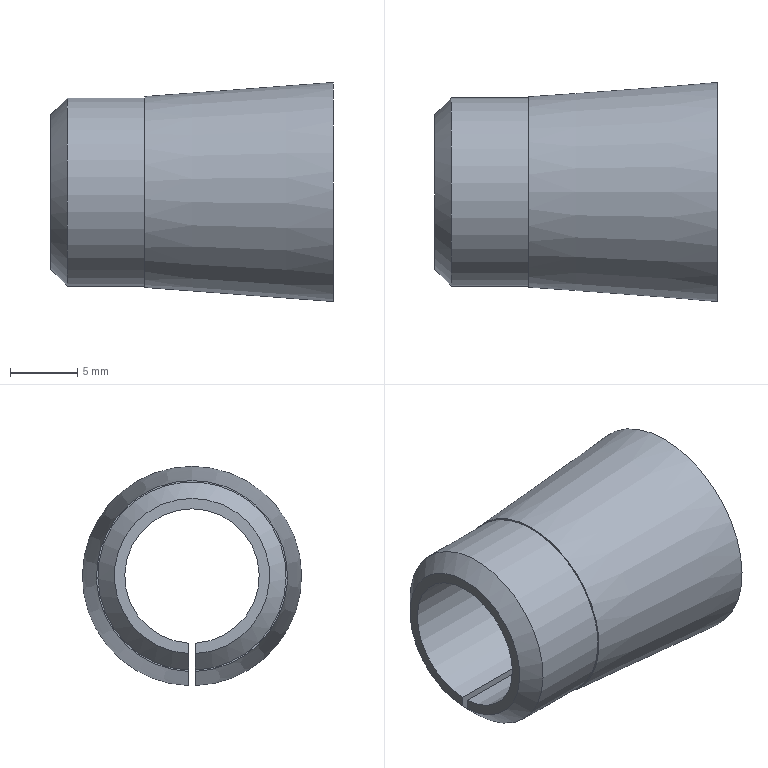Part | STEP file | 2_6 | 1 solid | 9 faces | box 21 x 16.3 x 16.296 mm | volume 1933 mm3 | plane 5 | cone 2 | cylinder 2 | commonest cylinder face diameters 10 x1 14 x1
STEP:
#1=CARTESIAN_POINT('',(0.,0.,0.));
#2=DIRECTION('',(0.,0.,1.));
#3=DIRECTION('',(1.,0.,0.));
#4=AXIS2_PLACEMENT_3D('',#1,#2,#3);
#5=CARTESIAN_POINT('',(7.,0.25,-7.096));
#6=VERTEX_POINT('',#5);
#7=CARTESIAN_POINT('',(7.,-0.25,-7.096));
#8=VERTEX_POINT('',#7);
#9=CARTESIAN_POINT('',(7.,0.,0.));
#10=DIRECTION('',(1.,0.,0.));
#11=DIRECTION('',(0.,0.,-1.));
#12=AXIS2_PLACEMENT_3D('',#9,#10,#11);
#13=CIRCLE('',#12,7.1);
#14=CARTESIAN_POINT('',(21.,0.,0.));
#15=DIRECTION('',(1.,0.,0.));
#16=DIRECTION('',(0.,0.,-1.));
#17=AXIS2_PLACEMENT_3D('',#14,#15,#16);
#18=CONICAL_SURFACE('',#17,8.15,0.07486);
#19=CARTESIAN_POINT('',(0.,-14.));
#20=DIRECTION('',(1.,0.));
#21=VECTOR('',#20,1.);
#22=LINE('',#19,#21);
#23=(GEOMETRIC_REPRESENTATION_CONTEXT(2)PARAMETRIC_REPRESENTATION_CONTEXT()REPRESENTATION_CONTEXT('',''));
#24=DEFINITIONAL_REPRESENTATION('',(#22),#23);
#25=PCURVE('',#18,#24);
#26=CARTESIAN_POINT('',(7.,7.05,0.));
#27=DIRECTION('',(-1.,0.,0.));
#28=DIRECTION('',(0.,0.,1.));
#29=AXIS2_PLACEMENT_3D('',#26,#27,#28);
#30=PLANE('',#29);
#31=CARTESIAN_POINT('',(-7.1,-7.05));
#32=CARTESIAN_POINT('',(-7.1,5.248));
#33=CARTESIAN_POINT('',(3.55,-0.9012));
#34=CARTESIAN_POINT('',(14.2,-7.05));
#35=CARTESIAN_POINT('',(3.55,-13.199));
#36=CARTESIAN_POINT('',(-7.1,-19.348));
#37=CARTESIAN_POINT('',(-7.1,-7.05));
#38=(BOUNDED_CURVE()B_SPLINE_CURVE(2,(#31,#32,#33,#34,#35,#36,#37),.UNSPECIFIED.,.T.,.F.)B_SPLINE_CURVE_WITH_KNOTS((1,2,2,2,2,1),(-2.094,0.,2.094,4.189,6.283,8.378),.UNSPECIFIED.)CURVE()GEOMETRIC_REPRESENTATION_ITEM()RATIONAL_B_SPLINE_CURVE((1.,0.5,1.,0.5,1.,0.5,1.))REPRESENTATION_ITEM(''));
#39=(GEOMETRIC_REPRESENTATION_CONTEXT(2)PARAMETRIC_REPRESENTATION_CONTEXT()REPRESENTATION_CONTEXT('',''));
#40=DEFINITIONAL_REPRESENTATION('',(#38),#39);
#41=PCURVE('',#30,#40);
#42=SURFACE_CURVE('',#13,(#25,#41),.PCURVE_S1.);
#43=EDGE_CURVE('',#6,#8,#42,.T.);
#44=ORIENTED_EDGE('',*,*,#43,.T.);
#45=CARTESIAN_POINT('',(21.,-0.25,-8.146));
#46=VERTEX_POINT('',#45);
#47=CARTESIAN_POINT('',(7.,-0.25,-7.096));
#48=CARTESIAN_POINT('',(11.667,-0.25,-7.446));
#49=CARTESIAN_POINT('',(16.333,-0.25,-7.796));
#50=CARTESIAN_POINT('',(21.,-0.25,-8.146));
#51=B_SPLINE_CURVE_WITH_KNOTS('',3,(#47,#48,#49,#50),.UNSPECIFIED.,.F.,.F.,(4,4),(0.,0.01404),.PIECEWISE_BEZIER_KNOTS.);
#52=CARTESIAN_POINT('',(6.248,-14.));
#53=CARTESIAN_POINT('',(6.248,-13.788));
#54=CARTESIAN_POINT('',(6.248,-13.364));
#55=CARTESIAN_POINT('',(6.248,-12.727));
#56=CARTESIAN_POINT('',(6.249,-12.091));
#57=CARTESIAN_POINT('',(6.249,-11.455));
#58=CARTESIAN_POINT('',(6.249,-10.818));
#59=CARTESIAN_POINT('',(6.249,-10.182));
#60=CARTESIAN_POINT('',(6.25,-9.545));
#61=CARTESIAN_POINT('',(6.25,-8.909));
#62=CARTESIAN_POINT('',(6.25,-8.273));
#63=CARTESIAN_POINT('',(6.25,-7.636));
#64=CARTESIAN_POINT('',(6.25,-7.));
#65=CARTESIAN_POINT('',(6.251,-6.364));
#66=CARTESIAN_POINT('',(6.251,-5.727));
#67=CARTESIAN_POINT('',(6.251,-5.091));
#68=CARTESIAN_POINT('',(6.251,-4.455));
#69=CARTESIAN_POINT('',(6.251,-3.818));
#70=CARTESIAN_POINT('',(6.252,-3.182));
#71=CARTESIAN_POINT('',(6.252,-2.545));
#72=CARTESIAN_POINT('',(6.252,-1.909));
#73=CARTESIAN_POINT('',(6.252,-1.273));
#74=CARTESIAN_POINT('',(6.252,-0.6364));
#75=CARTESIAN_POINT('',(6.252,-0.2121));
#76=CARTESIAN_POINT('',(6.253,0.));
#77=B_SPLINE_CURVE_WITH_KNOTS('',3,(#52,#53,#54,#55,#56,#57,#58,#59,#60,#61,#62,#63,#64,#65,#66,#67,#68,#69,#70,#71,#72,#73,#74,#75,#76),.UNSPECIFIED.,.F.,.F.,(4,1,1,1,1,1,1,1,1,1,1,1,1,1,1,1,1,1,1,1,1,1,4),(0.,0.0006382,0.001276,0.001914,0.002553,0.003191,0.003829,0.004467,0.005105,0.005743,0.006382,0.00702,0.007658,0.008296,0.008934,0.009572,0.01021,0.01085,0.01149,0.01212,0.01276,0.0134,0.01404),.QUASI_UNIFORM_KNOTS.);
#78=(GEOMETRIC_REPRESENTATION_CONTEXT(2)PARAMETRIC_REPRESENTATION_CONTEXT()REPRESENTATION_CONTEXT('',''));
#79=DEFINITIONAL_REPRESENTATION('',(#77),#78);
#80=PCURVE('',#18,#79);
#81=CARTESIAN_POINT('',(0.,-0.25,0.));
#82=DIRECTION('',(0.,1.,0.));
#83=DIRECTION('',(0.,0.,1.));
#84=AXIS2_PLACEMENT_3D('',#81,#82,#83);
#85=PLANE('',#84);
#86=CARTESIAN_POINT('',(-7.096,7.));
#87=CARTESIAN_POINT('',(-7.446,11.667));
#88=CARTESIAN_POINT('',(-7.796,16.333));
#89=CARTESIAN_POINT('',(-8.146,21.));
#90=B_SPLINE_CURVE_WITH_KNOTS('',3,(#86,#87,#88,#89),.UNSPECIFIED.,.F.,.F.,(4,4),(0.,0.01404),.PIECEWISE_BEZIER_KNOTS.);
#91=(GEOMETRIC_REPRESENTATION_CONTEXT(2)PARAMETRIC_REPRESENTATION_CONTEXT()REPRESENTATION_CONTEXT('',''));
#92=DEFINITIONAL_REPRESENTATION('',(#90),#91);
#93=PCURVE('',#85,#92);
#94=SURFACE_CURVE('',#51,(#80,#93),.PCURVE_S1.);
#95=EDGE_CURVE('',#8,#46,#94,.T.);
#96=ORIENTED_EDGE('',*,*,#95,.T.);
#97=CARTESIAN_POINT('',(21.,0.25,-8.146));
#98=VERTEX_POINT('',#97);
#99=CARTESIAN_POINT('',(21.,0.,0.));
#100=DIRECTION('',(-1.,0.,0.));
#101=DIRECTION('',(0.,0.,-1.));
#102=AXIS2_PLACEMENT_3D('',#99,#100,#101);
#103=CIRCLE('',#102,8.15);
#104=CARTESIAN_POINT('',(6.283,0.));
#105=DIRECTION('',(-1.,0.));
#106=VECTOR('',#105,1.);
#107=LINE('',#104,#106);
#108=(GEOMETRIC_REPRESENTATION_CONTEXT(2)PARAMETRIC_REPRESENTATION_CONTEXT()REPRESENTATION_CONTEXT('',''));
#109=DEFINITIONAL_REPRESENTATION('',(#107),#108);
#110=PCURVE('',#18,#109);
#111=CARTESIAN_POINT('',(21.,4.075,0.));
#112=DIRECTION('',(1.,0.,0.));
#113=DIRECTION('',(0.,0.,-1.));
#114=AXIS2_PLACEMENT_3D('',#111,#112,#113);
#115=PLANE('',#114);
#116=CARTESIAN_POINT('',(8.15,-4.075));
#117=CARTESIAN_POINT('',(8.15,-18.191));
#118=CARTESIAN_POINT('',(-4.075,-11.133));
#119=CARTESIAN_POINT('',(-16.3,-4.075));
#120=CARTESIAN_POINT('',(-4.075,2.983));
#121=CARTESIAN_POINT('',(8.15,10.041));
#122=CARTESIAN_POINT('',(8.15,-4.075));
#123=(BOUNDED_CURVE()B_SPLINE_CURVE(2,(#116,#117,#118,#119,#120,#121,#122),.UNSPECIFIED.,.T.,.F.)B_SPLINE_CURVE_WITH_KNOTS((1,2,2,2,2,1),(-2.094,0.,2.094,4.189,6.283,8.378),.UNSPECIFIED.)CURVE()GEOMETRIC_REPRESENTATION_ITEM()RATIONAL_B_SPLINE_CURVE((1.,0.5,1.,0.5,1.,0.5,1.))REPRESENTATION_ITEM(''));
#124=(GEOMETRIC_REPRESENTATION_CONTEXT(2)PARAMETRIC_REPRESENTATION_CONTEXT()REPRESENTATION_CONTEXT('',''));
#125=DEFINITIONAL_REPRESENTATION('',(#123),#124);
#126=PCURVE('',#115,#125);
#127=SURFACE_CURVE('',#103,(#110,#126),.PCURVE_S1.);
#128=EDGE_CURVE('',#46,#98,#127,.T.);
#129=ORIENTED_EDGE('',*,*,#128,.T.);
#130=CARTESIAN_POINT('',(21.,0.25,-8.146));
#131=CARTESIAN_POINT('',(16.333,0.25,-7.796));
#132=CARTESIAN_POINT('',(11.667,0.25,-7.446));
#133=CARTESIAN_POINT('',(7.,0.25,-7.096));
#134=B_SPLINE_CURVE_WITH_KNOTS('',3,(#130,#131,#132,#133),.UNSPECIFIED.,.F.,.F.,(4,4),(0.,0.01404),.PIECEWISE_BEZIER_KNOTS.);
#135=CARTESIAN_POINT('',(0.03068,0.));
#136=CARTESIAN_POINT('',(0.03074,-0.2121));
#137=CARTESIAN_POINT('',(0.03086,-0.6364));
#138=CARTESIAN_POINT('',(0.03104,-1.273));
#139=CARTESIAN_POINT('',(0.03123,-1.909));
#140=CARTESIAN_POINT('',(0.03142,-2.545));
#141=CARTESIAN_POINT('',(0.0316,-3.182));
#142=CARTESIAN_POINT('',(0.0318,-3.818));
#143=CARTESIAN_POINT('',(0.03199,-4.455));
#144=CARTESIAN_POINT('',(0.03219,-5.091));
#145=CARTESIAN_POINT('',(0.03239,-5.727));
#146=CARTESIAN_POINT('',(0.03259,-6.364));
#147=CARTESIAN_POINT('',(0.03279,-7.));
#148=CARTESIAN_POINT('',(0.033,-7.636));
#149=CARTESIAN_POINT('',(0.03321,-8.273));
#150=CARTESIAN_POINT('',(0.03342,-8.909));
#151=CARTESIAN_POINT('',(0.03363,-9.545));
#152=CARTESIAN_POINT('',(0.03385,-10.182));
#153=CARTESIAN_POINT('',(0.03407,-10.818));
#154=CARTESIAN_POINT('',(0.0343,-11.455));
#155=CARTESIAN_POINT('',(0.03452,-12.091));
#156=CARTESIAN_POINT('',(0.03475,-12.727));
#157=CARTESIAN_POINT('',(0.03498,-13.364));
#158=CARTESIAN_POINT('',(0.03514,-13.788));
#159=CARTESIAN_POINT('',(0.03522,-14.));
#160=B_SPLINE_CURVE_WITH_KNOTS('',3,(#135,#136,#137,#138,#139,#140,#141,#142,#143,#144,#145,#146,#147,#148,#149,#150,#151,#152,#153,#154,#155,#156,#157,#158,#159),.UNSPECIFIED.,.F.,.F.,(4,1,1,1,1,1,1,1,1,1,1,1,1,1,1,1,1,1,1,1,1,1,4),(0.,0.0006382,0.001276,0.001914,0.002553,0.003191,0.003829,0.004467,0.005105,0.005743,0.006382,0.00702,0.007658,0.008296,0.008934,0.009572,0.01021,0.01085,0.01149,0.01212,0.01276,0.0134,0.01404),.QUASI_UNIFORM_KNOTS.);
#161=(GEOMETRIC_REPRESENTATION_CONTEXT(2)PARAMETRIC_REPRESENTATION_CONTEXT()REPRESENTATION_CONTEXT('',''));
#162=DEFINITIONAL_REPRESENTATION('',(#160),#161);
#163=PCURVE('',#18,#162);
#164=CARTESIAN_POINT('',(0.,0.25,0.));
#165=DIRECTION('',(0.,1.,0.));
#166=DIRECTION('',(0.,0.,1.));
#167=AXIS2_PLACEMENT_3D('',#164,#165,#166);
#168=PLANE('',#167);
#169=CARTESIAN_POINT('',(-8.146,21.));
#170=CARTESIAN_POINT('',(-7.796,16.333));
#171=CARTESIAN_POINT('',(-7.446,11.667));
#172=CARTESIAN_POINT('',(-7.096,7.));
#173=B_SPLINE_CURVE_WITH_KNOTS('',3,(#169,#170,#171,#172),.UNSPECIFIED.,.F.,.F.,(4,4),(0.,0.01404),.PIECEWISE_BEZIER_KNOTS.);
#174=(GEOMETRIC_REPRESENTATION_CONTEXT(2)PARAMETRIC_REPRESENTATION_CONTEXT()REPRESENTATION_CONTEXT('',''));
#175=DEFINITIONAL_REPRESENTATION('',(#173),#174);
#176=PCURVE('',#168,#175);
#177=SURFACE_CURVE('',#134,(#163,#176),.PCURVE_S1.);
#178=EDGE_CURVE('',#98,#6,#177,.T.);
#179=ORIENTED_EDGE('',*,*,#178,.T.);
#180=EDGE_LOOP('',(#44,#96,#129,#179));
#181=FACE_BOUND('',#180,.T.);
#182=ADVANCED_FACE('',(#181),#18,.T.);
#183=ORIENTED_EDGE('',*,*,#128,.F.);
#184=CARTESIAN_POINT('',(21.,-0.25,-4.994));
#185=VERTEX_POINT('',#184);
#186=CARTESIAN_POINT('',(21.,-0.25,0.));
#187=DIRECTION('',(0.,0.,1.));
#188=VECTOR('',#187,1.);
#189=LINE('',#186,#188);
#190=CARTESIAN_POINT('',(0.,-4.325));
#191=DIRECTION('',(-1.,0.));
#192=VECTOR('',#191,1.);
#193=LINE('',#190,#192);
#194=(GEOMETRIC_REPRESENTATION_CONTEXT(2)PARAMETRIC_REPRESENTATION_CONTEXT()REPRESENTATION_CONTEXT('',''));
#195=DEFINITIONAL_REPRESENTATION('',(#193),#194);
#196=PCURVE('',#115,#195);
#197=CARTESIAN_POINT('',(0.,21.));
#198=DIRECTION('',(1.,0.));
#199=VECTOR('',#198,1.);
#200=LINE('',#197,#199);
#201=(GEOMETRIC_REPRESENTATION_CONTEXT(2)PARAMETRIC_REPRESENTATION_CONTEXT()REPRESENTATION_CONTEXT('',''));
#202=DEFINITIONAL_REPRESENTATION('',(#200),#201);
#203=PCURVE('',#85,#202);
#204=SURFACE_CURVE('',#189,(#196,#203),.PCURVE_S1.);
#205=EDGE_CURVE('',#46,#185,#204,.T.);
#206=ORIENTED_EDGE('',*,*,#205,.T.);
#207=CARTESIAN_POINT('',(21.,0.25,-4.994));
#208=VERTEX_POINT('',#207);
#209=CARTESIAN_POINT('',(21.,0.,0.));
#210=DIRECTION('',(-1.,0.,0.));
#211=DIRECTION('',(0.,0.,-1.));
#212=AXIS2_PLACEMENT_3D('',#209,#210,#211);
#213=CIRCLE('',#212,5.);
#214=CARTESIAN_POINT('',(5.,-4.075));
#215=CARTESIAN_POINT('',(5.,-12.735));
#216=CARTESIAN_POINT('',(-2.5,-8.405));
#217=CARTESIAN_POINT('',(-10.,-4.075));
#218=CARTESIAN_POINT('',(-2.5,0.2551));
#219=CARTESIAN_POINT('',(5.,4.585));
#220=CARTESIAN_POINT('',(5.,-4.075));
#221=(BOUNDED_CURVE()B_SPLINE_CURVE(2,(#214,#215,#216,#217,#218,#219,#220),.UNSPECIFIED.,.T.,.F.)B_SPLINE_CURVE_WITH_KNOTS((1,2,2,2,2,1),(-2.094,0.,2.094,4.189,6.283,8.378),.UNSPECIFIED.)CURVE()GEOMETRIC_REPRESENTATION_ITEM()RATIONAL_B_SPLINE_CURVE((1.,0.5,1.,0.5,1.,0.5,1.))REPRESENTATION_ITEM(''));
#222=(GEOMETRIC_REPRESENTATION_CONTEXT(2)PARAMETRIC_REPRESENTATION_CONTEXT()REPRESENTATION_CONTEXT('',''));
#223=DEFINITIONAL_REPRESENTATION('',(#221),#222);
#224=PCURVE('',#115,#223);
#225=CARTESIAN_POINT('',(10.5,0.,0.));
#226=DIRECTION('',(1.,0.,0.));
#227=DIRECTION('',(0.,0.,-1.));
#228=AXIS2_PLACEMENT_3D('',#225,#226,#227);
#229=CYLINDRICAL_SURFACE('',#228,5.);
#230=CARTESIAN_POINT('',(6.283,10.5));
#231=DIRECTION('',(-1.,0.));
#232=VECTOR('',#231,1.);
#233=LINE('',#230,#232);
#234=(GEOMETRIC_REPRESENTATION_CONTEXT(2)PARAMETRIC_REPRESENTATION_CONTEXT()REPRESENTATION_CONTEXT('',''));
#235=DEFINITIONAL_REPRESENTATION('',(#233),#234);
#236=PCURVE('',#229,#235);
#237=SURFACE_CURVE('',#213,(#224,#236),.PCURVE_S1.);
#238=EDGE_CURVE('',#185,#208,#237,.T.);
#239=ORIENTED_EDGE('',*,*,#238,.T.);
#240=CARTESIAN_POINT('',(21.,0.25,0.));
#241=DIRECTION('',(0.,0.,-1.));
#242=VECTOR('',#241,1.);
#243=LINE('',#240,#242);
#244=CARTESIAN_POINT('',(0.,-3.825));
#245=DIRECTION('',(1.,0.));
#246=VECTOR('',#245,1.);
#247=LINE('',#244,#246);
#248=(GEOMETRIC_REPRESENTATION_CONTEXT(2)PARAMETRIC_REPRESENTATION_CONTEXT()REPRESENTATION_CONTEXT('',''));
#249=DEFINITIONAL_REPRESENTATION('',(#247),#248);
#250=PCURVE('',#115,#249);
#251=CARTESIAN_POINT('',(0.,21.));
#252=DIRECTION('',(-1.,0.));
#253=VECTOR('',#252,1.);
#254=LINE('',#251,#253);
#255=(GEOMETRIC_REPRESENTATION_CONTEXT(2)PARAMETRIC_REPRESENTATION_CONTEXT()REPRESENTATION_CONTEXT('',''));
#256=DEFINITIONAL_REPRESENTATION('',(#254),#255);
#257=PCURVE('',#168,#256);
#258=SURFACE_CURVE('',#243,(#250,#257),.PCURVE_S1.);
#259=EDGE_CURVE('',#208,#98,#258,.T.);
#260=ORIENTED_EDGE('',*,*,#259,.T.);
#261=EDGE_LOOP('',(#183,#206,#239,#260));
#262=FACE_BOUND('',#261,.T.);
#263=ADVANCED_FACE('',(#262),#115,.T.);
#264=CARTESIAN_POINT('',(7.,0.25,-6.996));
#265=VERTEX_POINT('',#264);
#266=CARTESIAN_POINT('',(7.,0.25,0.));
#267=DIRECTION('',(0.,0.,1.));
#268=VECTOR('',#267,1.);
#269=LINE('',#266,#268);
#270=CARTESIAN_POINT('',(0.,-6.8));
#271=DIRECTION('',(1.,0.));
#272=VECTOR('',#271,1.);
#273=LINE('',#270,#272);
#274=(GEOMETRIC_REPRESENTATION_CONTEXT(2)PARAMETRIC_REPRESENTATION_CONTEXT()REPRESENTATION_CONTEXT('',''));
#275=DEFINITIONAL_REPRESENTATION('',(#273),#274);
#276=PCURVE('',#30,#275);
#277=CARTESIAN_POINT('',(0.,7.));
#278=DIRECTION('',(1.,0.));
#279=VECTOR('',#278,1.);
#280=LINE('',#277,#279);
#281=(GEOMETRIC_REPRESENTATION_CONTEXT(2)PARAMETRIC_REPRESENTATION_CONTEXT()REPRESENTATION_CONTEXT('',''));
#282=DEFINITIONAL_REPRESENTATION('',(#280),#281);
#283=PCURVE('',#168,#282);
#284=SURFACE_CURVE('',#269,(#276,#283),.PCURVE_S1.);
#285=EDGE_CURVE('',#6,#265,#284,.T.);
#286=ORIENTED_EDGE('',*,*,#285,.T.);
#287=CARTESIAN_POINT('',(7.,-0.25,-6.996));
#288=VERTEX_POINT('',#287);
#289=CARTESIAN_POINT('',(7.,0.,0.));
#290=DIRECTION('',(1.,0.,0.));
#291=DIRECTION('',(0.,0.,-1.));
#292=AXIS2_PLACEMENT_3D('',#289,#290,#291);
#293=CIRCLE('',#292,7.);
#294=CARTESIAN_POINT('',(-7.,-7.05));
#295=CARTESIAN_POINT('',(-7.,5.074));
#296=CARTESIAN_POINT('',(3.5,-0.9878));
#297=CARTESIAN_POINT('',(14.,-7.05));
#298=CARTESIAN_POINT('',(3.5,-13.112));
#299=CARTESIAN_POINT('',(-7.,-19.174));
#300=CARTESIAN_POINT('',(-7.,-7.05));
#301=(BOUNDED_CURVE()B_SPLINE_CURVE(2,(#294,#295,#296,#297,#298,#299,#300),.UNSPECIFIED.,.T.,.F.)B_SPLINE_CURVE_WITH_KNOTS((1,2,2,2,2,1),(-2.094,0.,2.094,4.189,6.283,8.378),.UNSPECIFIED.)CURVE()GEOMETRIC_REPRESENTATION_ITEM()RATIONAL_B_SPLINE_CURVE((1.,0.5,1.,0.5,1.,0.5,1.))REPRESENTATION_ITEM(''));
#302=(GEOMETRIC_REPRESENTATION_CONTEXT(2)PARAMETRIC_REPRESENTATION_CONTEXT()REPRESENTATION_CONTEXT('',''));
#303=DEFINITIONAL_REPRESENTATION('',(#301),#302);
#304=PCURVE('',#30,#303);
#305=CARTESIAN_POINT('',(4.114,0.,0.));
#306=DIRECTION('',(1.,0.,0.));
#307=DIRECTION('',(0.,0.,-1.));
#308=AXIS2_PLACEMENT_3D('',#305,#306,#307);
#309=CYLINDRICAL_SURFACE('',#308,7.);
#310=CARTESIAN_POINT('',(0.,2.886));
#311=DIRECTION('',(1.,0.));
#312=VECTOR('',#311,1.);
#313=LINE('',#310,#312);
#314=(GEOMETRIC_REPRESENTATION_CONTEXT(2)PARAMETRIC_REPRESENTATION_CONTEXT()REPRESENTATION_CONTEXT('',''));
#315=DEFINITIONAL_REPRESENTATION('',(#313),#314);
#316=PCURVE('',#309,#315);
#317=SURFACE_CURVE('',#293,(#304,#316),.PCURVE_S1.);
#318=EDGE_CURVE('',#265,#288,#317,.T.);
#319=ORIENTED_EDGE('',*,*,#318,.T.);
#320=CARTESIAN_POINT('',(7.,-0.25,0.));
#321=DIRECTION('',(0.,0.,-1.));
#322=VECTOR('',#321,1.);
#323=LINE('',#320,#322);
#324=CARTESIAN_POINT('',(0.,-7.3));
#325=DIRECTION('',(-1.,0.));
#326=VECTOR('',#325,1.);
#327=LINE('',#324,#326);
#328=(GEOMETRIC_REPRESENTATION_CONTEXT(2)PARAMETRIC_REPRESENTATION_CONTEXT()REPRESENTATION_CONTEXT('',''));
#329=DEFINITIONAL_REPRESENTATION('',(#327),#328);
#330=PCURVE('',#30,#329);
#331=CARTESIAN_POINT('',(0.,7.));
#332=DIRECTION('',(-1.,0.));
#333=VECTOR('',#332,1.);
#334=LINE('',#331,#333);
#335=(GEOMETRIC_REPRESENTATION_CONTEXT(2)PARAMETRIC_REPRESENTATION_CONTEXT()REPRESENTATION_CONTEXT('',''));
#336=DEFINITIONAL_REPRESENTATION('',(#334),#335);
#337=PCURVE('',#85,#336);
#338=SURFACE_CURVE('',#323,(#330,#337),.PCURVE_S1.);
#339=EDGE_CURVE('',#288,#8,#338,.T.);
#340=ORIENTED_EDGE('',*,*,#339,.T.);
#341=ORIENTED_EDGE('',*,*,#43,.F.);
#342=EDGE_LOOP('',(#286,#319,#340,#341));
#343=FACE_BOUND('',#342,.T.);
#344=ADVANCED_FACE('',(#343),#30,.T.);
#345=CARTESIAN_POINT('',(1.227,-0.25,-6.996));
#346=VERTEX_POINT('',#345);
#347=CARTESIAN_POINT('',(0.,-0.25,-5.768));
#348=VERTEX_POINT('',#347);
#349=CARTESIAN_POINT('',(1.227,-0.25,-6.996));
#350=CARTESIAN_POINT('',(0.818,-0.25,-6.586));
#351=CARTESIAN_POINT('',(0.409,-0.25,-6.177));
#352=CARTESIAN_POINT('',(0.,-0.25,-5.768));
#353=B_SPLINE_CURVE_WITH_KNOTS('',3,(#349,#350,#351,#352),.UNSPECIFIED.,.F.,.F.,(4,4),(0.,0.001736),.PIECEWISE_BEZIER_KNOTS.);
#354=CARTESIAN_POINT('',(-6.996,1.227));
#355=CARTESIAN_POINT('',(-6.586,0.818));
#356=CARTESIAN_POINT('',(-6.177,0.409));
#357=CARTESIAN_POINT('',(-5.768,0.));
#358=B_SPLINE_CURVE_WITH_KNOTS('',3,(#354,#355,#356,#357),.UNSPECIFIED.,.F.,.F.,(4,4),(0.,0.001736),.PIECEWISE_BEZIER_KNOTS.);
#359=(GEOMETRIC_REPRESENTATION_CONTEXT(2)PARAMETRIC_REPRESENTATION_CONTEXT()REPRESENTATION_CONTEXT('',''));
#360=DEFINITIONAL_REPRESENTATION('',(#358),#359);
#361=PCURVE('',#85,#360);
#362=CARTESIAN_POINT('',(1.227,0.,0.));
#363=DIRECTION('',(1.,0.,0.));
#364=DIRECTION('',(0.,0.,-1.));
#365=AXIS2_PLACEMENT_3D('',#362,#363,#364);
#366=CONICAL_SURFACE('',#365,7.,0.7854);
#367=CARTESIAN_POINT('',(6.247,0.));
#368=CARTESIAN_POINT('',(6.247,-0.01859));
#369=CARTESIAN_POINT('',(6.247,-0.05578));
#370=CARTESIAN_POINT('',(6.247,-0.1116));
#371=CARTESIAN_POINT('',(6.247,-0.1673));
#372=CARTESIAN_POINT('',(6.246,-0.2231));
#373=CARTESIAN_POINT('',(6.246,-0.2789));
#374=CARTESIAN_POINT('',(6.246,-0.3347));
#375=CARTESIAN_POINT('',(6.245,-0.3904));
#376=CARTESIAN_POINT('',(6.245,-0.4462));
#377=CARTESIAN_POINT('',(6.245,-0.502));
#378=CARTESIAN_POINT('',(6.244,-0.5577));
#379=CARTESIAN_POINT('',(6.244,-0.6135));
#380=CARTESIAN_POINT('',(6.244,-0.6693));
#381=CARTESIAN_POINT('',(6.243,-0.7251));
#382=CARTESIAN_POINT('',(6.243,-0.7808));
#383=CARTESIAN_POINT('',(6.243,-0.8366));
#384=CARTESIAN_POINT('',(6.242,-0.8924));
#385=CARTESIAN_POINT('',(6.242,-0.9482));
#386=CARTESIAN_POINT('',(6.241,-1.004));
#387=CARTESIAN_POINT('',(6.241,-1.06));
#388=CARTESIAN_POINT('',(6.241,-1.115));
#389=CARTESIAN_POINT('',(6.24,-1.171));
#390=CARTESIAN_POINT('',(6.24,-1.208));
#391=CARTESIAN_POINT('',(6.24,-1.227));
#392=B_SPLINE_CURVE_WITH_KNOTS('',3,(#367,#368,#369,#370,#371,#372,#373,#374,#375,#376,#377,#378,#379,#380,#381,#382,#383,#384,#385,#386,#387,#388,#389,#390,#391),.UNSPECIFIED.,.F.,.F.,(4,1,1,1,1,1,1,1,1,1,1,1,1,1,1,1,1,1,1,1,1,1,4),(0.,0.00007891,0.0001578,0.0002367,0.0003156,0.0003945,0.0004734,0.0005523,0.0006312,0.0007101,0.0007891,0.000868,0.0009469,0.001026,0.001105,0.001184,0.001262,0.001341,0.00142,0.001499,0.001578,0.001657,0.001736),.QUASI_UNIFORM_KNOTS.);
#393=(GEOMETRIC_REPRESENTATION_CONTEXT(2)PARAMETRIC_REPRESENTATION_CONTEXT()REPRESENTATION_CONTEXT('',''));
#394=DEFINITIONAL_REPRESENTATION('',(#392),#393);
#395=PCURVE('',#366,#394);
#396=SURFACE_CURVE('',#353,(#361,#395),.PCURVE_S1.);
#397=EDGE_CURVE('',#346,#348,#396,.T.);
#398=ORIENTED_EDGE('',*,*,#397,.T.);
#399=CARTESIAN_POINT('',(0.,-0.25,-4.994));
#400=VERTEX_POINT('',#399);
#401=CARTESIAN_POINT('',(0.,-0.25,0.));
#402=DIRECTION('',(0.,0.,-1.));
#403=VECTOR('',#402,1.);
#404=LINE('',#401,#403);
#405=CARTESIAN_POINT('',(0.,0.));
#406=DIRECTION('',(-1.,0.));
#407=VECTOR('',#406,1.);
#408=LINE('',#405,#407);
#409=(GEOMETRIC_REPRESENTATION_CONTEXT(2)PARAMETRIC_REPRESENTATION_CONTEXT()REPRESENTATION_CONTEXT('',''));
#410=DEFINITIONAL_REPRESENTATION('',(#408),#409);
#411=PCURVE('',#85,#410);
#412=CARTESIAN_POINT('',(0.,2.886,0.));
#413=DIRECTION('',(-1.,0.,0.));
#414=DIRECTION('',(0.,0.,1.));
#415=AXIS2_PLACEMENT_3D('',#412,#413,#414);
#416=PLANE('',#415);
#417=CARTESIAN_POINT('',(0.,-3.136));
#418=DIRECTION('',(-1.,0.));
#419=VECTOR('',#418,1.);
#420=LINE('',#417,#419);
#421=(GEOMETRIC_REPRESENTATION_CONTEXT(2)PARAMETRIC_REPRESENTATION_CONTEXT()REPRESENTATION_CONTEXT('',''));
#422=DEFINITIONAL_REPRESENTATION('',(#420),#421);
#423=PCURVE('',#416,#422);
#424=SURFACE_CURVE('',#404,(#411,#423),.PCURVE_S1.);
#425=EDGE_CURVE('',#400,#348,#424,.T.);
#426=ORIENTED_EDGE('',*,*,#425,.F.);
#427=CARTESIAN_POINT('',(0.,-0.25,-4.994));
#428=DIRECTION('',(1.,0.,0.));
#429=VECTOR('',#428,1.);
#430=LINE('',#427,#429);
#431=CARTESIAN_POINT('',(-4.994,0.));
#432=DIRECTION('',(0.,1.));
#433=VECTOR('',#432,1.);
#434=LINE('',#431,#433);
#435=(GEOMETRIC_REPRESENTATION_CONTEXT(2)PARAMETRIC_REPRESENTATION_CONTEXT()REPRESENTATION_CONTEXT('',''));
#436=DEFINITIONAL_REPRESENTATION('',(#434),#435);
#437=PCURVE('',#85,#436);
#438=CARTESIAN_POINT('',(6.233,-10.5));
#439=DIRECTION('',(0.,1.));
#440=VECTOR('',#439,1.);
#441=LINE('',#438,#440);
#442=(GEOMETRIC_REPRESENTATION_CONTEXT(2)PARAMETRIC_REPRESENTATION_CONTEXT()REPRESENTATION_CONTEXT('',''));
#443=DEFINITIONAL_REPRESENTATION('',(#441),#442);
#444=PCURVE('',#229,#443);
#445=SURFACE_CURVE('',#430,(#437,#444),.PCURVE_S1.);
#446=EDGE_CURVE('',#400,#185,#445,.T.);
#447=ORIENTED_EDGE('',*,*,#446,.T.);
#448=ORIENTED_EDGE('',*,*,#205,.F.);
#449=ORIENTED_EDGE('',*,*,#95,.F.);
#450=ORIENTED_EDGE('',*,*,#339,.F.);
#451=CARTESIAN_POINT('',(0.,-0.25,-6.996));
#452=DIRECTION('',(-1.,0.,0.));
#453=VECTOR('',#452,1.);
#454=LINE('',#451,#453);
#455=CARTESIAN_POINT('',(-6.996,0.));
#456=DIRECTION('',(0.,-1.));
#457=VECTOR('',#456,1.);
#458=LINE('',#455,#457);
#459=(GEOMETRIC_REPRESENTATION_CONTEXT(2)PARAMETRIC_REPRESENTATION_CONTEXT()REPRESENTATION_CONTEXT('',''));
#460=DEFINITIONAL_REPRESENTATION('',(#458),#459);
#461=PCURVE('',#85,#460);
#462=CARTESIAN_POINT('',(6.247,-4.114));
#463=DIRECTION('',(0.,-1.));
#464=VECTOR('',#463,1.);
#465=LINE('',#462,#464);
#466=(GEOMETRIC_REPRESENTATION_CONTEXT(2)PARAMETRIC_REPRESENTATION_CONTEXT()REPRESENTATION_CONTEXT('',''));
#467=DEFINITIONAL_REPRESENTATION('',(#465),#466);
#468=PCURVE('',#309,#467);
#469=SURFACE_CURVE('',#454,(#461,#468),.PCURVE_S1.);
#470=EDGE_CURVE('',#288,#346,#469,.T.);
#471=ORIENTED_EDGE('',*,*,#470,.T.);
#472=EDGE_LOOP('',(#398,#426,#447,#448,#449,#450,#471));
#473=FACE_BOUND('',#472,.T.);
#474=ADVANCED_FACE('',(#473),#85,.T.);
#475=CARTESIAN_POINT('',(0.,0.25,-5.768));
#476=VERTEX_POINT('',#475);
#477=CARTESIAN_POINT('',(0.,0.25,-4.994));
#478=VERTEX_POINT('',#477);
#479=CARTESIAN_POINT('',(0.,0.25,0.));
#480=DIRECTION('',(0.,0.,1.));
#481=VECTOR('',#480,1.);
#482=LINE('',#479,#481);
#483=CARTESIAN_POINT('',(0.,0.));
#484=DIRECTION('',(1.,0.));
#485=VECTOR('',#484,1.);
#486=LINE('',#483,#485);
#487=(GEOMETRIC_REPRESENTATION_CONTEXT(2)PARAMETRIC_REPRESENTATION_CONTEXT()REPRESENTATION_CONTEXT('',''));
#488=DEFINITIONAL_REPRESENTATION('',(#486),#487);
#489=PCURVE('',#168,#488);
#490=CARTESIAN_POINT('',(0.,-2.636));
#491=DIRECTION('',(1.,0.));
#492=VECTOR('',#491,1.);
#493=LINE('',#490,#492);
#494=(GEOMETRIC_REPRESENTATION_CONTEXT(2)PARAMETRIC_REPRESENTATION_CONTEXT()REPRESENTATION_CONTEXT('',''));
#495=DEFINITIONAL_REPRESENTATION('',(#493),#494);
#496=PCURVE('',#416,#495);
#497=SURFACE_CURVE('',#482,(#489,#496),.PCURVE_S1.);
#498=EDGE_CURVE('',#476,#478,#497,.T.);
#499=ORIENTED_EDGE('',*,*,#498,.F.);
#500=CARTESIAN_POINT('',(1.227,0.25,-6.996));
#501=VERTEX_POINT('',#500);
#502=CARTESIAN_POINT('',(1.227,0.25,-6.996));
#503=CARTESIAN_POINT('',(0.818,0.25,-6.586));
#504=CARTESIAN_POINT('',(0.409,0.25,-6.177));
#505=CARTESIAN_POINT('',(0.,0.25,-5.768));
#506=B_SPLINE_CURVE_WITH_KNOTS('',3,(#502,#503,#504,#505),.UNSPECIFIED.,.F.,.F.,(4,4),(0.,0.001736),.PIECEWISE_BEZIER_KNOTS.);
#507=CARTESIAN_POINT('',(-6.996,1.227));
#508=CARTESIAN_POINT('',(-6.586,0.818));
#509=CARTESIAN_POINT('',(-6.177,0.409));
#510=CARTESIAN_POINT('',(-5.768,0.));
#511=B_SPLINE_CURVE_WITH_KNOTS('',3,(#507,#508,#509,#510),.UNSPECIFIED.,.F.,.F.,(4,4),(0.,0.001736),.PIECEWISE_BEZIER_KNOTS.);
#512=(GEOMETRIC_REPRESENTATION_CONTEXT(2)PARAMETRIC_REPRESENTATION_CONTEXT()REPRESENTATION_CONTEXT('',''));
#513=DEFINITIONAL_REPRESENTATION('',(#511),#512);
#514=PCURVE('',#168,#513);
#515=CARTESIAN_POINT('',(0.03572,0.));
#516=CARTESIAN_POINT('',(0.03582,-0.01859));
#517=CARTESIAN_POINT('',(0.03601,-0.05578));
#518=CARTESIAN_POINT('',(0.0363,-0.1116));
#519=CARTESIAN_POINT('',(0.0366,-0.1673));
#520=CARTESIAN_POINT('',(0.0369,-0.2231));
#521=CARTESIAN_POINT('',(0.0372,-0.2789));
#522=CARTESIAN_POINT('',(0.03752,-0.3347));
#523=CARTESIAN_POINT('',(0.03783,-0.3904));
#524=CARTESIAN_POINT('',(0.03815,-0.4462));
#525=CARTESIAN_POINT('',(0.03848,-0.502));
#526=CARTESIAN_POINT('',(0.03882,-0.5577));
#527=CARTESIAN_POINT('',(0.03915,-0.6135));
#528=CARTESIAN_POINT('',(0.0395,-0.6693));
#529=CARTESIAN_POINT('',(0.03985,-0.7251));
#530=CARTESIAN_POINT('',(0.04021,-0.7808));
#531=CARTESIAN_POINT('',(0.04057,-0.8366));
#532=CARTESIAN_POINT('',(0.04094,-0.8924));
#533=CARTESIAN_POINT('',(0.04132,-0.9482));
#534=CARTESIAN_POINT('',(0.0417,-1.004));
#535=CARTESIAN_POINT('',(0.0421,-1.06));
#536=CARTESIAN_POINT('',(0.0425,-1.115));
#537=CARTESIAN_POINT('',(0.0429,-1.171));
#538=CARTESIAN_POINT('',(0.04318,-1.208));
#539=CARTESIAN_POINT('',(0.04332,-1.227));
#540=B_SPLINE_CURVE_WITH_KNOTS('',3,(#515,#516,#517,#518,#519,#520,#521,#522,#523,#524,#525,#526,#527,#528,#529,#530,#531,#532,#533,#534,#535,#536,#537,#538,#539),.UNSPECIFIED.,.F.,.F.,(4,1,1,1,1,1,1,1,1,1,1,1,1,1,1,1,1,1,1,1,1,1,4),(0.,0.00007891,0.0001578,0.0002367,0.0003156,0.0003945,0.0004734,0.0005523,0.0006312,0.0007101,0.0007891,0.000868,0.0009469,0.001026,0.001105,0.001184,0.001262,0.001341,0.00142,0.001499,0.001578,0.001657,0.001736),.QUASI_UNIFORM_KNOTS.);
#541=(GEOMETRIC_REPRESENTATION_CONTEXT(2)PARAMETRIC_REPRESENTATION_CONTEXT()REPRESENTATION_CONTEXT('',''));
#542=DEFINITIONAL_REPRESENTATION('',(#540),#541);
#543=PCURVE('',#366,#542);
#544=SURFACE_CURVE('',#506,(#514,#543),.PCURVE_S1.);
#545=EDGE_CURVE('',#501,#476,#544,.T.);
#546=ORIENTED_EDGE('',*,*,#545,.F.);
#547=CARTESIAN_POINT('',(0.,0.25,-6.996));
#548=DIRECTION('',(-1.,0.,0.));
#549=VECTOR('',#548,1.);
#550=LINE('',#547,#549);
#551=CARTESIAN_POINT('',(-6.996,0.));
#552=DIRECTION('',(0.,-1.));
#553=VECTOR('',#552,1.);
#554=LINE('',#551,#553);
#555=(GEOMETRIC_REPRESENTATION_CONTEXT(2)PARAMETRIC_REPRESENTATION_CONTEXT()REPRESENTATION_CONTEXT('',''));
#556=DEFINITIONAL_REPRESENTATION('',(#554),#555);
#557=PCURVE('',#168,#556);
#558=CARTESIAN_POINT('',(0.03572,-4.114));
#559=DIRECTION('',(0.,-1.));
#560=VECTOR('',#559,1.);
#561=LINE('',#558,#560);
#562=(GEOMETRIC_REPRESENTATION_CONTEXT(2)PARAMETRIC_REPRESENTATION_CONTEXT()REPRESENTATION_CONTEXT('',''));
#563=DEFINITIONAL_REPRESENTATION('',(#561),#562);
#564=PCURVE('',#309,#563);
#565=SURFACE_CURVE('',#550,(#557,#564),.PCURVE_S1.);
#566=EDGE_CURVE('',#265,#501,#565,.T.);
#567=ORIENTED_EDGE('',*,*,#566,.F.);
#568=ORIENTED_EDGE('',*,*,#285,.F.);
#569=ORIENTED_EDGE('',*,*,#178,.F.);
#570=ORIENTED_EDGE('',*,*,#259,.F.);
#571=CARTESIAN_POINT('',(0.,0.25,-4.994));
#572=DIRECTION('',(1.,0.,0.));
#573=VECTOR('',#572,1.);
#574=LINE('',#571,#573);
#575=CARTESIAN_POINT('',(-4.994,0.));
#576=DIRECTION('',(0.,1.));
#577=VECTOR('',#576,1.);
#578=LINE('',#575,#577);
#579=(GEOMETRIC_REPRESENTATION_CONTEXT(2)PARAMETRIC_REPRESENTATION_CONTEXT()REPRESENTATION_CONTEXT('',''));
#580=DEFINITIONAL_REPRESENTATION('',(#578),#579);
#581=PCURVE('',#168,#580);
#582=CARTESIAN_POINT('',(0.05002,-10.5));
#583=DIRECTION('',(0.,1.));
#584=VECTOR('',#583,1.);
#585=LINE('',#582,#584);
#586=(GEOMETRIC_REPRESENTATION_CONTEXT(2)PARAMETRIC_REPRESENTATION_CONTEXT()REPRESENTATION_CONTEXT('',''));
#587=DEFINITIONAL_REPRESENTATION('',(#585),#586);
#588=PCURVE('',#229,#587);
#589=SURFACE_CURVE('',#574,(#581,#588),.PCURVE_S1.);
#590=EDGE_CURVE('',#478,#208,#589,.T.);
#591=ORIENTED_EDGE('',*,*,#590,.F.);
#592=EDGE_LOOP('',(#499,#546,#567,#568,#569,#570,#591));
#593=FACE_BOUND('',#592,.T.);
#594=ADVANCED_FACE('',(#593),#168,.F.);
#595=ORIENTED_EDGE('',*,*,#446,.T.);
#596=ORIENTED_EDGE('',*,*,#238,.T.);
#597=ORIENTED_EDGE('',*,*,#590,.F.);
#598=CARTESIAN_POINT('',(0.,0.,0.));
#599=DIRECTION('',(1.,0.,0.));
#600=DIRECTION('',(0.,0.,-1.));
#601=AXIS2_PLACEMENT_3D('',#598,#599,#600);
#602=CIRCLE('',#601,5.);
#603=CARTESIAN_POINT('',(0.,-10.5));
#604=DIRECTION('',(1.,0.));
#605=VECTOR('',#604,1.);
#606=LINE('',#603,#605);
#607=(GEOMETRIC_REPRESENTATION_CONTEXT(2)PARAMETRIC_REPRESENTATION_CONTEXT()REPRESENTATION_CONTEXT('',''));
#608=DEFINITIONAL_REPRESENTATION('',(#606),#607);
#609=PCURVE('',#229,#608);
#610=CARTESIAN_POINT('',(-5.,-2.886));
#611=CARTESIAN_POINT('',(-5.,5.774));
#612=CARTESIAN_POINT('',(2.5,1.444));
#613=CARTESIAN_POINT('',(10.,-2.886));
#614=CARTESIAN_POINT('',(2.5,-7.217));
#615=CARTESIAN_POINT('',(-5.,-11.547));
#616=CARTESIAN_POINT('',(-5.,-2.886));
#617=(BOUNDED_CURVE()B_SPLINE_CURVE(2,(#610,#611,#612,#613,#614,#615,#616),.UNSPECIFIED.,.T.,.F.)B_SPLINE_CURVE_WITH_KNOTS((1,2,2,2,2,1),(-2.094,0.,2.094,4.189,6.283,8.378),.UNSPECIFIED.)CURVE()GEOMETRIC_REPRESENTATION_ITEM()RATIONAL_B_SPLINE_CURVE((1.,0.5,1.,0.5,1.,0.5,1.))REPRESENTATION_ITEM(''));
#618=(GEOMETRIC_REPRESENTATION_CONTEXT(2)PARAMETRIC_REPRESENTATION_CONTEXT()REPRESENTATION_CONTEXT('',''));
#619=DEFINITIONAL_REPRESENTATION('',(#617),#618);
#620=PCURVE('',#416,#619);
#621=SURFACE_CURVE('',#602,(#609,#620),.PCURVE_S1.);
#622=EDGE_CURVE('',#478,#400,#621,.T.);
#623=ORIENTED_EDGE('',*,*,#622,.T.);
#624=EDGE_LOOP('',(#595,#596,#597,#623));
#625=FACE_BOUND('',#624,.F.);
#626=ADVANCED_FACE('',(#625),#229,.F.);
#627=ORIENTED_EDGE('',*,*,#470,.F.);
#628=ORIENTED_EDGE('',*,*,#318,.F.);
#629=ORIENTED_EDGE('',*,*,#566,.T.);
#630=CARTESIAN_POINT('',(1.227,0.,0.));
#631=DIRECTION('',(1.,0.,0.));
#632=DIRECTION('',(0.,0.,-1.));
#633=AXIS2_PLACEMENT_3D('',#630,#631,#632);
#634=CIRCLE('',#633,7.);
#635=CARTESIAN_POINT('',(0.,-2.886));
#636=DIRECTION('',(1.,0.));
#637=VECTOR('',#636,1.);
#638=LINE('',#635,#637);
#639=(GEOMETRIC_REPRESENTATION_CONTEXT(2)PARAMETRIC_REPRESENTATION_CONTEXT()REPRESENTATION_CONTEXT('',''));
#640=DEFINITIONAL_REPRESENTATION('',(#638),#639);
#641=PCURVE('',#309,#640);
#642=CARTESIAN_POINT('',(0.,0.));
#643=DIRECTION('',(1.,0.));
#644=VECTOR('',#643,1.);
#645=LINE('',#642,#644);
#646=(GEOMETRIC_REPRESENTATION_CONTEXT(2)PARAMETRIC_REPRESENTATION_CONTEXT()REPRESENTATION_CONTEXT('',''));
#647=DEFINITIONAL_REPRESENTATION('',(#645),#646);
#648=PCURVE('',#366,#647);
#649=SURFACE_CURVE('',#634,(#641,#648),.PCURVE_S1.);
#650=EDGE_CURVE('',#501,#346,#649,.T.);
#651=ORIENTED_EDGE('',*,*,#650,.T.);
#652=EDGE_LOOP('',(#627,#628,#629,#651));
#653=FACE_BOUND('',#652,.T.);
#654=ADVANCED_FACE('',(#653),#309,.T.);
#655=ORIENTED_EDGE('',*,*,#397,.F.);
#656=ORIENTED_EDGE('',*,*,#650,.F.);
#657=ORIENTED_EDGE('',*,*,#545,.T.);
#658=CARTESIAN_POINT('',(0.,0.,0.));
#659=DIRECTION('',(1.,0.,0.));
#660=DIRECTION('',(0.,0.,-1.));
#661=AXIS2_PLACEMENT_3D('',#658,#659,#660);
#662=CIRCLE('',#661,5.773);
#663=CARTESIAN_POINT('',(0.,-1.227));
#664=DIRECTION('',(1.,0.));
#665=VECTOR('',#664,1.);
#666=LINE('',#663,#665);
#667=(GEOMETRIC_REPRESENTATION_CONTEXT(2)PARAMETRIC_REPRESENTATION_CONTEXT()REPRESENTATION_CONTEXT('',''));
#668=DEFINITIONAL_REPRESENTATION('',(#666),#667);
#669=PCURVE('',#366,#668);
#670=CARTESIAN_POINT('',(-5.773,-2.886));
#671=CARTESIAN_POINT('',(-5.773,7.113));
#672=CARTESIAN_POINT('',(2.887,2.113));
#673=CARTESIAN_POINT('',(11.546,-2.886));
#674=CARTESIAN_POINT('',(2.887,-7.886));
#675=CARTESIAN_POINT('',(-5.773,-12.886));
#676=CARTESIAN_POINT('',(-5.773,-2.886));
#677=(BOUNDED_CURVE()B_SPLINE_CURVE(2,(#670,#671,#672,#673,#674,#675,#676),.UNSPECIFIED.,.T.,.F.)B_SPLINE_CURVE_WITH_KNOTS((1,2,2,2,2,1),(-2.094,0.,2.094,4.189,6.283,8.378),.UNSPECIFIED.)CURVE()GEOMETRIC_REPRESENTATION_ITEM()RATIONAL_B_SPLINE_CURVE((1.,0.5,1.,0.5,1.,0.5,1.))REPRESENTATION_ITEM(''));
#678=(GEOMETRIC_REPRESENTATION_CONTEXT(2)PARAMETRIC_REPRESENTATION_CONTEXT()REPRESENTATION_CONTEXT('',''));
#679=DEFINITIONAL_REPRESENTATION('',(#677),#678);
#680=PCURVE('',#416,#679);
#681=SURFACE_CURVE('',#662,(#669,#680),.PCURVE_S1.);
#682=EDGE_CURVE('',#476,#348,#681,.T.);
#683=ORIENTED_EDGE('',*,*,#682,.T.);
#684=EDGE_LOOP('',(#655,#656,#657,#683));
#685=FACE_BOUND('',#684,.T.);
#686=ADVANCED_FACE('',(#685),#366,.T.);
#687=ORIENTED_EDGE('',*,*,#682,.F.);
#688=ORIENTED_EDGE('',*,*,#498,.T.);
#689=ORIENTED_EDGE('',*,*,#622,.T.);
#690=ORIENTED_EDGE('',*,*,#425,.T.);
#691=EDGE_LOOP('',(#687,#688,#689,#690));
#692=FACE_BOUND('',#691,.T.);
#693=ADVANCED_FACE('',(#692),#416,.T.);
#694=CLOSED_SHELL('',(#182,#263,#344,#474,#594,#626,#654,#686,#693));
#695=MANIFOLD_SOLID_BREP('',#694);
#696=(LENGTH_UNIT()NAMED_UNIT(*)SI_UNIT(.MILLI.,.METRE.));
#697=UNCERTAINTY_MEASURE_WITH_UNIT(LENGTH_MEASURE(0.0000002),#696,'','');
#698=(NAMED_UNIT(*)PLANE_ANGLE_UNIT()SI_UNIT($,.RADIAN.));
#699=(NAMED_UNIT(*)SI_UNIT($,.STERADIAN.)SOLID_ANGLE_UNIT());
#700=(GEOMETRIC_REPRESENTATION_CONTEXT(3)GLOBAL_UNCERTAINTY_ASSIGNED_CONTEXT((#697))GLOBAL_UNIT_ASSIGNED_CONTEXT((#696,#698,#699))REPRESENTATION_CONTEXT('',''));
#701=ADVANCED_BREP_SHAPE_REPRESENTATION('',(#4,#695),#700);